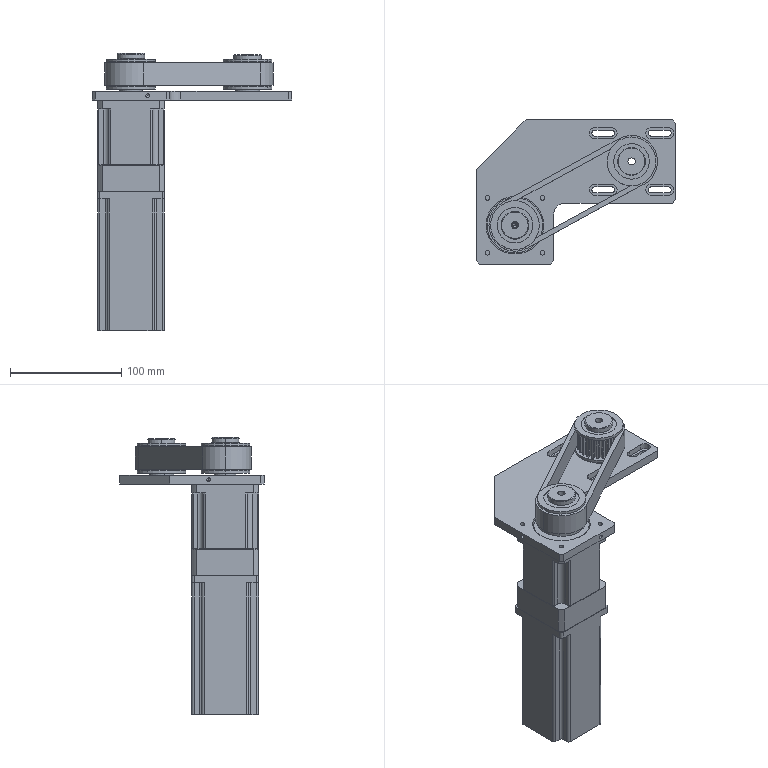Part | SolidWorks | 10 solids | 598 faces | box 180 x 130 x 249.5 mm | volume 881824 mm3 | plane 282 | cylinder 266 | cone 38 | torus 12 | commonest cylinder face diameters 38.65 x52 5.5 x28 4 x26 3.3 x16 10 x16 5 x13